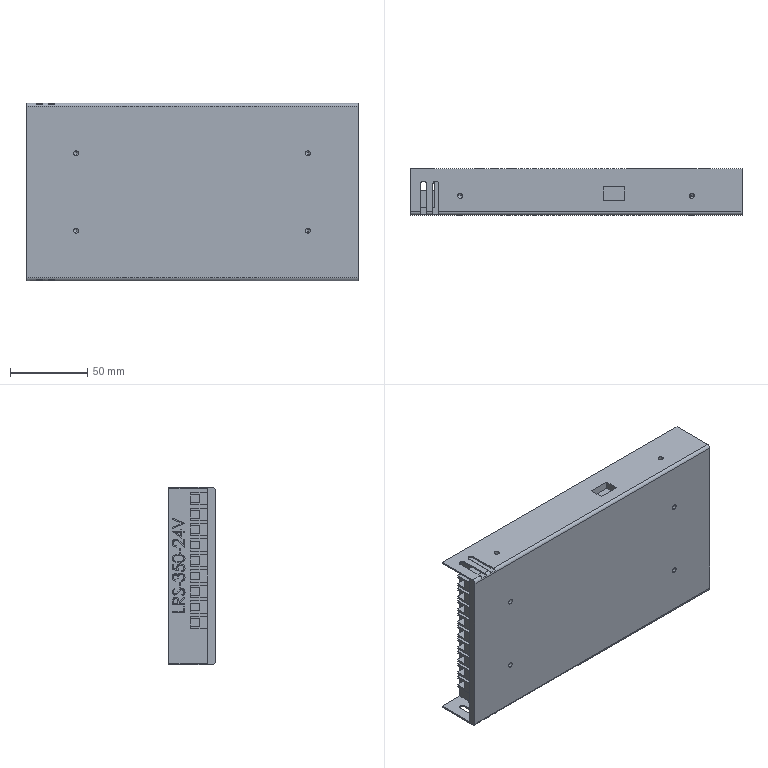Part | STEP file | Switching power supply LRS-350-24 | 11 solids | 416 faces | box 215 x 30 x 115 mm | volume 695683 mm3 | plane 239 | cylinder 104 | spline 57 | cone 16 | commonest cylinder face diameters 5 x60 3.3 x16 4 x6 25 x5 35 x5 45 x5